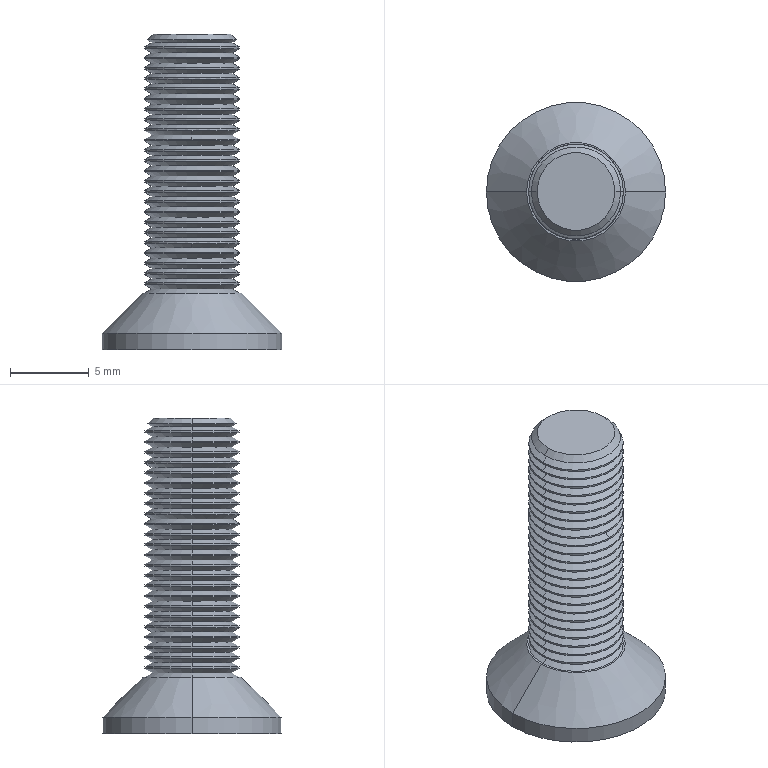Part | SolidWorks | features BaseBody 1 | 1 solid | 171 faces | box 11.34 x 11.34 x 20 mm | volume 634.609 mm3 | cone 106 | cylinder 50 | plane 15 | commonest cylinder face diameters 6 x48 11.34 x2